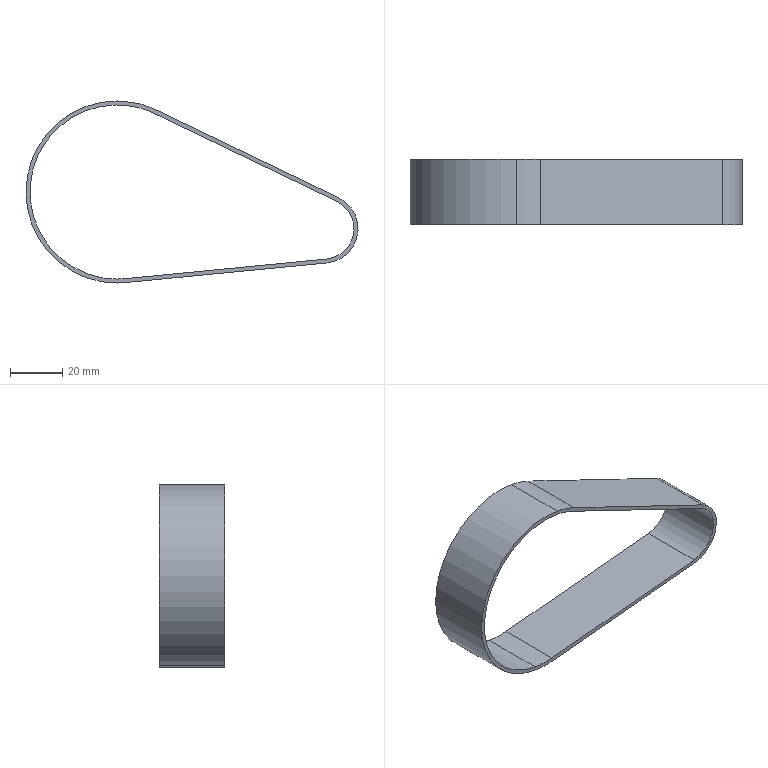Part | SolidWorks | features BaseBody 1 | 1 solid | 14 faces | box 127.707 x 25 x 70 mm | volume 11936 mm3 | cylinder 8 | plane 6 | commonest cylinder face diameters 66.96 x3 70 x3 23.46 x1 26.5 x1
STEP:
#1=CARTESIAN_POINT('',(1958.854,161.2,885.964));
#2=VERTEX_POINT('',#1);
#3=CARTESIAN_POINT('',(1947.146,161.2,820.036));
#4=VERTEX_POINT('',#3);
#5=CARTESIAN_POINT('',(1953.,161.2,853.));
#6=DIRECTION('',(0.,-1.,0.));
#7=DIRECTION('',(0.4337,0.,0.901));
#8=AXIS2_PLACEMENT_3D('',#5,#6,#7);
#9=CIRCLE('',#8,33.48);
#10=EDGE_CURVE('',#2,#4,#9,.T.);
#11=ORIENTED_EDGE('',*,*,#10,.T.);
#12=CARTESIAN_POINT('',(1947.146,186.2,820.036));
#13=VERTEX_POINT('',#12);
#14=CARTESIAN_POINT('',(1947.146,161.2,820.036));
#15=DIRECTION('',(0.,1.,0.));
#16=VECTOR('',#15,1000.);
#17=LINE('',#14,#16);
#18=EDGE_CURVE('',#4,#13,#17,.T.);
#19=ORIENTED_EDGE('',*,*,#18,.T.);
#20=CARTESIAN_POINT('',(1958.854,186.2,885.964));
#21=VERTEX_POINT('',#20);
#22=CARTESIAN_POINT('',(1953.,186.2,853.));
#23=DIRECTION('',(0.,-1.,0.));
#24=DIRECTION('',(0.4337,0.,0.901));
#25=AXIS2_PLACEMENT_3D('',#22,#23,#24);
#26=CIRCLE('',#25,33.48);
#27=EDGE_CURVE('',#21,#13,#26,.T.);
#28=ORIENTED_EDGE('',*,*,#27,.F.);
#29=CARTESIAN_POINT('',(1958.854,161.2,885.964));
#30=DIRECTION('',(0.,1.,0.));
#31=VECTOR('',#30,1000.);
#32=LINE('',#29,#31);
#33=EDGE_CURVE('',#2,#21,#32,.T.);
#34=ORIENTED_EDGE('',*,*,#33,.F.);
#35=EDGE_LOOP('',(#11,#19,#28,#34));
#36=FACE_OUTER_BOUND('',#35,.T.);
#37=CARTESIAN_POINT('',(1953.,161.2,853.));
#38=DIRECTION('',(0.,1.,0.));
#39=DIRECTION('',(0.1749,0.,0.9846));
#40=AXIS2_PLACEMENT_3D('',#37,#38,#39);
#41=CYLINDRICAL_SURFACE('',#40,33.48);
#42=ADVANCED_FACE('',(#36),#41,.F.);
#43=CARTESIAN_POINT('',(1967.522,161.2,883.167));
#44=VERTEX_POINT('',#43);
#45=CARTESIAN_POINT('',(1953.,161.2,853.));
#46=DIRECTION('',(0.,-1.,0.));
#47=DIRECTION('',(0.4337,0.,0.901));
#48=AXIS2_PLACEMENT_3D('',#45,#46,#47);
#49=CIRCLE('',#48,33.48);
#50=EDGE_CURVE('',#44,#2,#49,.T.);
#51=ORIENTED_EDGE('',*,*,#50,.T.);
#52=ORIENTED_EDGE('',*,*,#33,.T.);
#53=CARTESIAN_POINT('',(1967.522,186.2,883.167));
#54=VERTEX_POINT('',#53);
#55=CARTESIAN_POINT('',(1953.,186.2,853.));
#56=DIRECTION('',(0.,-1.,0.));
#57=DIRECTION('',(0.4337,0.,0.901));
#58=AXIS2_PLACEMENT_3D('',#55,#56,#57);
#59=CIRCLE('',#58,33.48);
#60=EDGE_CURVE('',#54,#21,#59,.T.);
#61=ORIENTED_EDGE('',*,*,#60,.F.);
#62=CARTESIAN_POINT('',(1967.522,161.2,883.167));
#63=DIRECTION('',(0.,1.,0.));
#64=VECTOR('',#63,1000.);
#65=LINE('',#62,#64);
#66=EDGE_CURVE('',#44,#54,#65,.T.);
#67=ORIENTED_EDGE('',*,*,#66,.F.);
#68=EDGE_LOOP('',(#51,#52,#61,#67));
#69=FACE_OUTER_BOUND('',#68,.T.);
#70=CARTESIAN_POINT('',(1953.,161.2,853.));
#71=DIRECTION('',(0.,1.,0.));
#72=DIRECTION('',(0.1749,0.,0.9846));
#73=AXIS2_PLACEMENT_3D('',#70,#71,#72);
#74=CYLINDRICAL_SURFACE('',#73,33.48);
#75=ADVANCED_FACE('',(#69),#74,.F.);
#76=CARTESIAN_POINT('',(1956.394,161.2,818.165));
#77=VERTEX_POINT('',#76);
#78=CARTESIAN_POINT('',(1946.88,161.2,818.539));
#79=VERTEX_POINT('',#78);
#80=CARTESIAN_POINT('',(1953.,161.2,853.));
#81=DIRECTION('',(0.,1.,0.));
#82=DIRECTION('',(0.09698,0.,-0.9953));
#83=AXIS2_PLACEMENT_3D('',#80,#81,#82);
#84=CIRCLE('',#83,35.);
#85=EDGE_CURVE('',#77,#79,#84,.T.);
#86=ORIENTED_EDGE('',*,*,#85,.T.);
#87=CARTESIAN_POINT('',(1946.88,186.2,818.539));
#88=VERTEX_POINT('',#87);
#89=CARTESIAN_POINT('',(1946.88,161.2,818.539));
#90=DIRECTION('',(0.,1.,0.));
#91=VECTOR('',#90,1000.);
#92=LINE('',#89,#91);
#93=EDGE_CURVE('',#79,#88,#92,.T.);
#94=ORIENTED_EDGE('',*,*,#93,.T.);
#95=CARTESIAN_POINT('',(1956.394,186.2,818.165));
#96=VERTEX_POINT('',#95);
#97=CARTESIAN_POINT('',(1953.,186.2,853.));
#98=DIRECTION('',(0.,1.,0.));
#99=DIRECTION('',(0.09698,0.,-0.9953));
#100=AXIS2_PLACEMENT_3D('',#97,#98,#99);
#101=CIRCLE('',#100,35.);
#102=EDGE_CURVE('',#96,#88,#101,.T.);
#103=ORIENTED_EDGE('',*,*,#102,.F.);
#104=CARTESIAN_POINT('',(1956.394,161.2,818.165));
#105=DIRECTION('',(0.,1.,0.));
#106=VECTOR('',#105,1000.);
#107=LINE('',#104,#106);
#108=EDGE_CURVE('',#77,#96,#107,.T.);
#109=ORIENTED_EDGE('',*,*,#108,.F.);
#110=EDGE_LOOP('',(#86,#94,#103,#109));
#111=FACE_OUTER_BOUND('',#110,.T.);
#112=CARTESIAN_POINT('',(1953.,161.2,853.));
#113=DIRECTION('',(0.,1.,0.));
#114=DIRECTION('',(0.1749,0.,0.9846));
#115=AXIS2_PLACEMENT_3D('',#112,#113,#114);
#116=CYLINDRICAL_SURFACE('',#115,35.);
#117=ADVANCED_FACE('',(#111),#116,.T.);
#118=ORIENTED_EDGE('',*,*,#93,.F.);
#119=CARTESIAN_POINT('',(1959.12,161.2,887.461));
#120=VERTEX_POINT('',#119);
#121=CARTESIAN_POINT('',(1953.,161.2,853.));
#122=DIRECTION('',(0.,1.,0.));
#123=DIRECTION('',(0.09698,0.,-0.9953));
#124=AXIS2_PLACEMENT_3D('',#121,#122,#123);
#125=CIRCLE('',#124,35.);
#126=EDGE_CURVE('',#79,#120,#125,.T.);
#127=ORIENTED_EDGE('',*,*,#126,.T.);
#128=CARTESIAN_POINT('',(1959.12,186.2,887.461));
#129=VERTEX_POINT('',#128);
#130=CARTESIAN_POINT('',(1959.12,161.2,887.461));
#131=DIRECTION('',(0.,1.,0.));
#132=VECTOR('',#131,1000.);
#133=LINE('',#130,#132);
#134=EDGE_CURVE('',#120,#129,#133,.T.);
#135=ORIENTED_EDGE('',*,*,#134,.T.);
#136=CARTESIAN_POINT('',(1953.,186.2,853.));
#137=DIRECTION('',(0.,1.,0.));
#138=DIRECTION('',(0.09698,0.,-0.9953));
#139=AXIS2_PLACEMENT_3D('',#136,#137,#138);
#140=CIRCLE('',#139,35.);
#141=EDGE_CURVE('',#88,#129,#140,.T.);
#142=ORIENTED_EDGE('',*,*,#141,.F.);
#143=EDGE_LOOP('',(#118,#127,#135,#142));
#144=FACE_OUTER_BOUND('',#143,.T.);
#145=CARTESIAN_POINT('',(1953.,161.2,853.));
#146=DIRECTION('',(0.,1.,0.));
#147=DIRECTION('',(0.1749,0.,0.9846));
#148=AXIS2_PLACEMENT_3D('',#145,#146,#147);
#149=CYLINDRICAL_SURFACE('',#148,35.);
#150=ADVANCED_FACE('',(#144),#149,.T.);
#151=CARTESIAN_POINT('',(1968.181,161.2,884.536));
#152=VERTEX_POINT('',#151);
#153=CARTESIAN_POINT('',(2038.204,161.2,850.828));
#154=VERTEX_POINT('',#153);
#155=CARTESIAN_POINT('',(1968.181,161.2,884.536));
#156=DIRECTION('',(0.901,0.,-0.4337));
#157=VECTOR('',#156,1000.);
#158=LINE('',#155,#157);
#159=EDGE_CURVE('',#152,#154,#158,.T.);
#160=ORIENTED_EDGE('',*,*,#159,.F.);
#161=CARTESIAN_POINT('',(1953.,161.2,853.));
#162=DIRECTION('',(0.,1.,0.));
#163=DIRECTION('',(0.09698,0.,-0.9953));
#164=AXIS2_PLACEMENT_3D('',#161,#162,#163);
#165=CIRCLE('',#164,35.);
#166=EDGE_CURVE('',#120,#152,#165,.T.);
#167=ORIENTED_EDGE('',*,*,#166,.F.);
#168=ORIENTED_EDGE('',*,*,#126,.F.);
#169=ORIENTED_EDGE('',*,*,#85,.F.);
#170=CARTESIAN_POINT('',(2033.742,161.2,825.702));
#171=VERTEX_POINT('',#170);
#172=CARTESIAN_POINT('',(2033.742,161.2,825.702));
#173=DIRECTION('',(-0.9953,0.,-0.09698));
#174=VECTOR('',#173,1000.);
#175=LINE('',#172,#174);
#176=EDGE_CURVE('',#171,#77,#175,.T.);
#177=ORIENTED_EDGE('',*,*,#176,.F.);
#178=CARTESIAN_POINT('',(2032.457,161.2,838.889));
#179=DIRECTION('',(0.,1.,0.));
#180=DIRECTION('',(0.4337,0.,0.901));
#181=AXIS2_PLACEMENT_3D('',#178,#179,#180);
#182=CIRCLE('',#181,13.25);
#183=EDGE_CURVE('',#154,#171,#182,.T.);
#184=ORIENTED_EDGE('',*,*,#183,.F.);
#185=EDGE_LOOP('',(#160,#167,#168,#169,#177,#184));
#186=FACE_OUTER_BOUND('',#185,.T.);
#187=CARTESIAN_POINT('',(2037.545,161.2,849.459));
#188=VERTEX_POINT('',#187);
#189=CARTESIAN_POINT('',(2037.545,161.2,849.459));
#190=DIRECTION('',(-0.901,0.,0.4337));
#191=VECTOR('',#190,1000.);
#192=LINE('',#189,#191);
#193=EDGE_CURVE('',#188,#44,#192,.T.);
#194=ORIENTED_EDGE('',*,*,#193,.F.);
#195=CARTESIAN_POINT('',(2033.594,161.2,827.215));
#196=VERTEX_POINT('',#195);
#197=CARTESIAN_POINT('',(2032.457,161.2,838.889));
#198=DIRECTION('',(0.,-1.,0.));
#199=DIRECTION('',(0.09698,0.,-0.9953));
#200=AXIS2_PLACEMENT_3D('',#197,#198,#199);
#201=CIRCLE('',#200,11.73);
#202=EDGE_CURVE('',#196,#188,#201,.T.);
#203=ORIENTED_EDGE('',*,*,#202,.F.);
#204=CARTESIAN_POINT('',(1956.247,161.2,819.678));
#205=VERTEX_POINT('',#204);
#206=CARTESIAN_POINT('',(1956.247,161.2,819.678));
#207=DIRECTION('',(0.9953,0.,0.09698));
#208=VECTOR('',#207,1000.);
#209=LINE('',#206,#208);
#210=EDGE_CURVE('',#205,#196,#209,.T.);
#211=ORIENTED_EDGE('',*,*,#210,.F.);
#212=CARTESIAN_POINT('',(1953.,161.2,853.));
#213=DIRECTION('',(0.,-1.,0.));
#214=DIRECTION('',(0.4337,0.,0.901));
#215=AXIS2_PLACEMENT_3D('',#212,#213,#214);
#216=CIRCLE('',#215,33.48);
#217=EDGE_CURVE('',#4,#205,#216,.T.);
#218=ORIENTED_EDGE('',*,*,#217,.F.);
#219=ORIENTED_EDGE('',*,*,#10,.F.);
#220=ORIENTED_EDGE('',*,*,#50,.F.);
#221=EDGE_LOOP('',(#194,#203,#211,#218,#219,#220));
#222=FACE_BOUND('',#221,.T.);
#223=CARTESIAN_POINT('',(1953.,161.2,853.));
#224=DIRECTION('',(0.,1.,0.));
#225=DIRECTION('',(0.1749,0.,0.9846));
#226=AXIS2_PLACEMENT_3D('',#223,#224,#225);
#227=PLANE('',#226);
#228=ADVANCED_FACE('',(#186,#222),#227,.F.);
#229=CARTESIAN_POINT('',(2033.742,186.2,825.702));
#230=VERTEX_POINT('',#229);
#231=CARTESIAN_POINT('',(2033.742,161.2,825.702));
#232=DIRECTION('',(0.,1.,0.));
#233=VECTOR('',#232,1000.);
#234=LINE('',#231,#233);
#235=EDGE_CURVE('',#171,#230,#234,.T.);
#236=ORIENTED_EDGE('',*,*,#235,.T.);
#237=CARTESIAN_POINT('',(2038.204,186.2,850.828));
#238=VERTEX_POINT('',#237);
#239=CARTESIAN_POINT('',(2032.457,186.2,838.889));
#240=DIRECTION('',(0.,1.,0.));
#241=DIRECTION('',(0.4337,0.,0.901));
#242=AXIS2_PLACEMENT_3D('',#239,#240,#241);
#243=CIRCLE('',#242,13.25);
#244=EDGE_CURVE('',#238,#230,#243,.T.);
#245=ORIENTED_EDGE('',*,*,#244,.F.);
#246=CARTESIAN_POINT('',(2038.204,161.2,850.828));
#247=DIRECTION('',(0.,1.,0.));
#248=VECTOR('',#247,1000.);
#249=LINE('',#246,#248);
#250=EDGE_CURVE('',#154,#238,#249,.T.);
#251=ORIENTED_EDGE('',*,*,#250,.F.);
#252=ORIENTED_EDGE('',*,*,#183,.T.);
#253=EDGE_LOOP('',(#236,#245,#251,#252));
#254=FACE_OUTER_BOUND('',#253,.T.);
#255=CARTESIAN_POINT('',(2032.457,161.2,838.889));
#256=DIRECTION('',(0.,1.,0.));
#257=DIRECTION('',(0.1749,0.,0.9846));
#258=AXIS2_PLACEMENT_3D('',#255,#256,#257);
#259=CYLINDRICAL_SURFACE('',#258,13.25);
#260=ADVANCED_FACE('',(#254),#259,.T.);
#261=ORIENTED_EDGE('',*,*,#250,.T.);
#262=CARTESIAN_POINT('',(1968.181,186.2,884.536));
#263=VERTEX_POINT('',#262);
#264=CARTESIAN_POINT('',(1968.181,186.2,884.536));
#265=DIRECTION('',(0.901,0.,-0.4337));
#266=VECTOR('',#265,1000.);
#267=LINE('',#264,#266);
#268=EDGE_CURVE('',#263,#238,#267,.T.);
#269=ORIENTED_EDGE('',*,*,#268,.F.);
#270=CARTESIAN_POINT('',(1968.181,161.2,884.536));
#271=DIRECTION('',(0.,1.,0.));
#272=VECTOR('',#271,1000.);
#273=LINE('',#270,#272);
#274=EDGE_CURVE('',#152,#263,#273,.T.);
#275=ORIENTED_EDGE('',*,*,#274,.F.);
#276=ORIENTED_EDGE('',*,*,#159,.T.);
#277=EDGE_LOOP('',(#261,#269,#275,#276));
#278=FACE_OUTER_BOUND('',#277,.T.);
#279=CARTESIAN_POINT('',(1968.181,161.2,884.536));
#280=DIRECTION('',(0.4337,0.,0.901));
#281=DIRECTION('',(0.901,0.,-0.4337));
#282=AXIS2_PLACEMENT_3D('',#279,#280,#281);
#283=PLANE('',#282);
#284=ADVANCED_FACE('',(#278),#283,.T.);
#285=ORIENTED_EDGE('',*,*,#134,.F.);
#286=ORIENTED_EDGE('',*,*,#166,.T.);
#287=ORIENTED_EDGE('',*,*,#274,.T.);
#288=CARTESIAN_POINT('',(1953.,186.2,853.));
#289=DIRECTION('',(0.,1.,0.));
#290=DIRECTION('',(0.09698,0.,-0.9953));
#291=AXIS2_PLACEMENT_3D('',#288,#289,#290);
#292=CIRCLE('',#291,35.);
#293=EDGE_CURVE('',#129,#263,#292,.T.);
#294=ORIENTED_EDGE('',*,*,#293,.F.);
#295=EDGE_LOOP('',(#285,#286,#287,#294));
#296=FACE_OUTER_BOUND('',#295,.T.);
#297=CARTESIAN_POINT('',(1953.,161.2,853.));
#298=DIRECTION('',(0.,1.,0.));
#299=DIRECTION('',(0.1749,0.,0.9846));
#300=AXIS2_PLACEMENT_3D('',#297,#298,#299);
#301=CYLINDRICAL_SURFACE('',#300,35.);
#302=ADVANCED_FACE('',(#296),#301,.T.);
#303=ORIENTED_EDGE('',*,*,#108,.T.);
#304=CARTESIAN_POINT('',(2033.742,186.2,825.702));
#305=DIRECTION('',(-0.9953,0.,-0.09698));
#306=VECTOR('',#305,1000.);
#307=LINE('',#304,#306);
#308=EDGE_CURVE('',#230,#96,#307,.T.);
#309=ORIENTED_EDGE('',*,*,#308,.F.);
#310=ORIENTED_EDGE('',*,*,#235,.F.);
#311=ORIENTED_EDGE('',*,*,#176,.T.);
#312=EDGE_LOOP('',(#303,#309,#310,#311));
#313=FACE_OUTER_BOUND('',#312,.T.);
#314=CARTESIAN_POINT('',(2033.742,161.2,825.702));
#315=DIRECTION('',(0.09698,0.,-0.9953));
#316=DIRECTION('',(-0.9953,0.,-0.09698));
#317=AXIS2_PLACEMENT_3D('',#314,#315,#316);
#318=PLANE('',#317);
#319=ADVANCED_FACE('',(#313),#318,.T.);
#320=ORIENTED_EDGE('',*,*,#308,.T.);
#321=ORIENTED_EDGE('',*,*,#102,.T.);
#322=ORIENTED_EDGE('',*,*,#141,.T.);
#323=ORIENTED_EDGE('',*,*,#293,.T.);
#324=ORIENTED_EDGE('',*,*,#268,.T.);
#325=ORIENTED_EDGE('',*,*,#244,.T.);
#326=EDGE_LOOP('',(#320,#321,#322,#323,#324,#325));
#327=FACE_OUTER_BOUND('',#326,.T.);
#328=CARTESIAN_POINT('',(1956.247,186.2,819.678));
#329=VERTEX_POINT('',#328);
#330=CARTESIAN_POINT('',(2033.594,186.2,827.215));
#331=VERTEX_POINT('',#330);
#332=CARTESIAN_POINT('',(1956.247,186.2,819.678));
#333=DIRECTION('',(0.9953,0.,0.09698));
#334=VECTOR('',#333,1000.);
#335=LINE('',#332,#334);
#336=EDGE_CURVE('',#329,#331,#335,.T.);
#337=ORIENTED_EDGE('',*,*,#336,.T.);
#338=CARTESIAN_POINT('',(2037.545,186.2,849.459));
#339=VERTEX_POINT('',#338);
#340=CARTESIAN_POINT('',(2032.457,186.2,838.889));
#341=DIRECTION('',(0.,-1.,0.));
#342=DIRECTION('',(0.09698,0.,-0.9953));
#343=AXIS2_PLACEMENT_3D('',#340,#341,#342);
#344=CIRCLE('',#343,11.73);
#345=EDGE_CURVE('',#331,#339,#344,.T.);
#346=ORIENTED_EDGE('',*,*,#345,.T.);
#347=CARTESIAN_POINT('',(2037.545,186.2,849.459));
#348=DIRECTION('',(-0.901,0.,0.4337));
#349=VECTOR('',#348,1000.);
#350=LINE('',#347,#349);
#351=EDGE_CURVE('',#339,#54,#350,.T.);
#352=ORIENTED_EDGE('',*,*,#351,.T.);
#353=ORIENTED_EDGE('',*,*,#60,.T.);
#354=ORIENTED_EDGE('',*,*,#27,.T.);
#355=CARTESIAN_POINT('',(1953.,186.2,853.));
#356=DIRECTION('',(0.,-1.,0.));
#357=DIRECTION('',(0.4337,0.,0.901));
#358=AXIS2_PLACEMENT_3D('',#355,#356,#357);
#359=CIRCLE('',#358,33.48);
#360=EDGE_CURVE('',#13,#329,#359,.T.);
#361=ORIENTED_EDGE('',*,*,#360,.T.);
#362=EDGE_LOOP('',(#337,#346,#352,#353,#354,#361));
#363=FACE_BOUND('',#362,.T.);
#364=CARTESIAN_POINT('',(1953.,186.2,853.));
#365=DIRECTION('',(0.,1.,0.));
#366=DIRECTION('',(0.1749,0.,0.9846));
#367=AXIS2_PLACEMENT_3D('',#364,#365,#366);
#368=PLANE('',#367);
#369=ADVANCED_FACE('',(#327,#363),#368,.T.);
#370=ORIENTED_EDGE('',*,*,#18,.F.);
#371=ORIENTED_EDGE('',*,*,#217,.T.);
#372=CARTESIAN_POINT('',(1956.247,161.2,819.678));
#373=DIRECTION('',(0.,1.,0.));
#374=VECTOR('',#373,1000.);
#375=LINE('',#372,#374);
#376=EDGE_CURVE('',#205,#329,#375,.T.);
#377=ORIENTED_EDGE('',*,*,#376,.T.);
#378=ORIENTED_EDGE('',*,*,#360,.F.);
#379=EDGE_LOOP('',(#370,#371,#377,#378));
#380=FACE_OUTER_BOUND('',#379,.T.);
#381=CARTESIAN_POINT('',(1953.,161.2,853.));
#382=DIRECTION('',(0.,1.,0.));
#383=DIRECTION('',(0.1749,0.,0.9846));
#384=AXIS2_PLACEMENT_3D('',#381,#382,#383);
#385=CYLINDRICAL_SURFACE('',#384,33.48);
#386=ADVANCED_FACE('',(#380),#385,.F.);
#387=ORIENTED_EDGE('',*,*,#66,.T.);
#388=ORIENTED_EDGE('',*,*,#351,.F.);
#389=CARTESIAN_POINT('',(2037.545,161.2,849.459));
#390=DIRECTION('',(0.,1.,0.));
#391=VECTOR('',#390,1000.);
#392=LINE('',#389,#391);
#393=EDGE_CURVE('',#188,#339,#392,.T.);
#394=ORIENTED_EDGE('',*,*,#393,.F.);
#395=ORIENTED_EDGE('',*,*,#193,.T.);
#396=EDGE_LOOP('',(#387,#388,#394,#395));
#397=FACE_OUTER_BOUND('',#396,.T.);
#398=CARTESIAN_POINT('',(2037.545,161.2,849.459));
#399=DIRECTION('',(-0.4337,0.,-0.901));
#400=DIRECTION('',(-0.901,0.,0.4337));
#401=AXIS2_PLACEMENT_3D('',#398,#399,#400);
#402=PLANE('',#401);
#403=ADVANCED_FACE('',(#397),#402,.T.);
#404=ORIENTED_EDGE('',*,*,#393,.T.);
#405=ORIENTED_EDGE('',*,*,#345,.F.);
#406=CARTESIAN_POINT('',(2033.594,161.2,827.215));
#407=DIRECTION('',(0.,1.,0.));
#408=VECTOR('',#407,1000.);
#409=LINE('',#406,#408);
#410=EDGE_CURVE('',#196,#331,#409,.T.);
#411=ORIENTED_EDGE('',*,*,#410,.F.);
#412=ORIENTED_EDGE('',*,*,#202,.T.);
#413=EDGE_LOOP('',(#404,#405,#411,#412));
#414=FACE_OUTER_BOUND('',#413,.T.);
#415=CARTESIAN_POINT('',(2032.457,161.2,838.889));
#416=DIRECTION('',(0.,1.,0.));
#417=DIRECTION('',(0.1749,0.,0.9846));
#418=AXIS2_PLACEMENT_3D('',#415,#416,#417);
#419=CYLINDRICAL_SURFACE('',#418,11.73);
#420=ADVANCED_FACE('',(#414),#419,.F.);
#421=ORIENTED_EDGE('',*,*,#410,.T.);
#422=ORIENTED_EDGE('',*,*,#336,.F.);
#423=ORIENTED_EDGE('',*,*,#376,.F.);
#424=ORIENTED_EDGE('',*,*,#210,.T.);
#425=EDGE_LOOP('',(#421,#422,#423,#424));
#426=FACE_OUTER_BOUND('',#425,.T.);
#427=CARTESIAN_POINT('',(1956.247,161.2,819.678));
#428=DIRECTION('',(-0.09698,0.,0.9953));
#429=DIRECTION('',(0.9953,0.,0.09698));
#430=AXIS2_PLACEMENT_3D('',#427,#428,#429);
#431=PLANE('',#430);
#432=ADVANCED_FACE('',(#426),#431,.T.);
#433=CLOSED_SHELL('',(#42,#75,#117,#150,#228,#260,#284,#302,#319,#369,#386,#403,#420,#432));
#434=MANIFOLD_SOLID_BREP('',#433);
#435=CARTESIAN_POINT('',(0.,0.,0.));
#436=DIRECTION('',(0.,0.,1.));
#437=DIRECTION('',(1.,0.,0.));
#438=AXIS2_PLACEMENT_3D('',#435,#436,#437);
#439=(LENGTH_UNIT()NAMED_UNIT(*)SI_UNIT(.MILLI.,.METRE.));
#440=UNCERTAINTY_MEASURE_WITH_UNIT(LENGTH_MEASURE(0.00001),#439,'','');
#441=(NAMED_UNIT(*)PLANE_ANGLE_UNIT()SI_UNIT($,.RADIAN.));
#442=(NAMED_UNIT(*)SI_UNIT($,.STERADIAN.)SOLID_ANGLE_UNIT());
#443=(GEOMETRIC_REPRESENTATION_CONTEXT(3)GLOBAL_UNCERTAINTY_ASSIGNED_CONTEXT((#440))GLOBAL_UNIT_ASSIGNED_CONTEXT((#439,#441,#442))REPRESENTATION_CONTEXT('',''));
#444=ADVANCED_BREP_SHAPE_REPRESENTATION('',(#434,#438),#443);